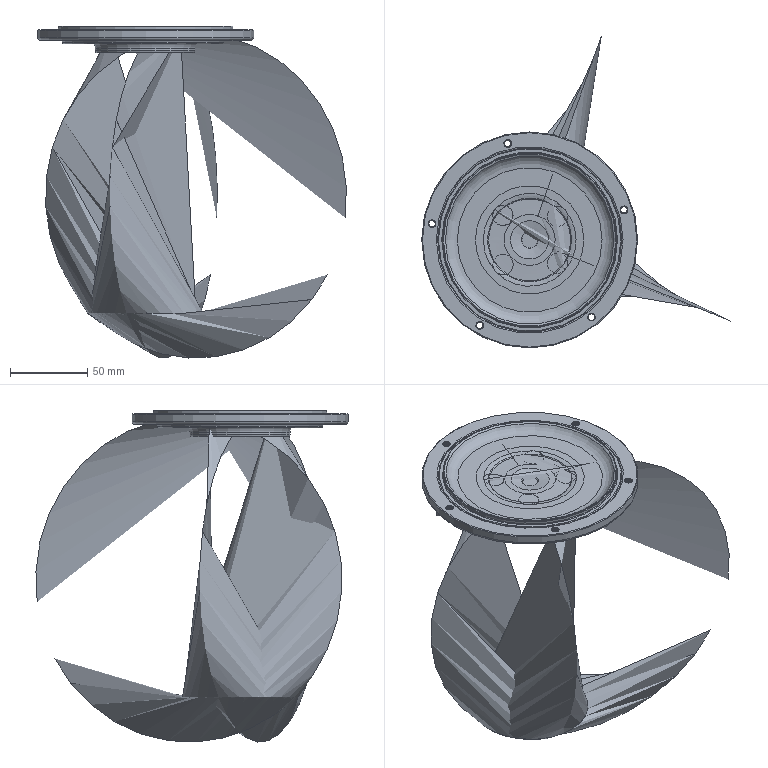Part | 2 solids | 160 faces | volume 15372714 mm3 | torus 45 | cylinder 42 | cone 26 | spline 25 | plane 22 | commonest cylinder face diameters 4.2 x21 5 x5 6.6 x4 13.1 x4 5.6 x2 10.002 x2